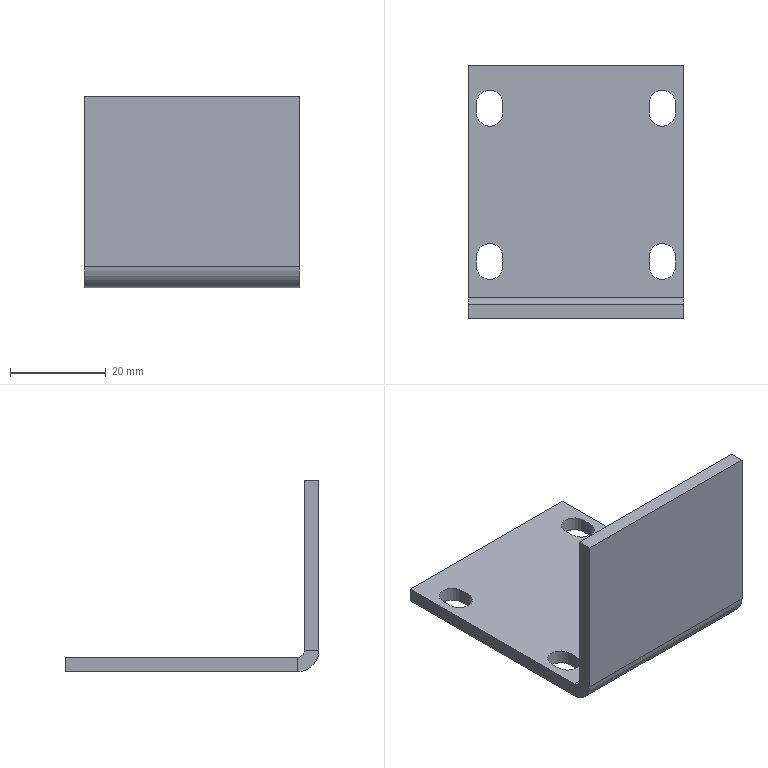Part | STEP file | Push-film plate (2) SGN-3-10 | 1 solid | 30 faces | box 45 x 53 x 40 mm | volume 11559 mm3 | plane 20 | cylinder 10 | commonest cylinder face diameters 5.5 x8 3 x1 9 x1